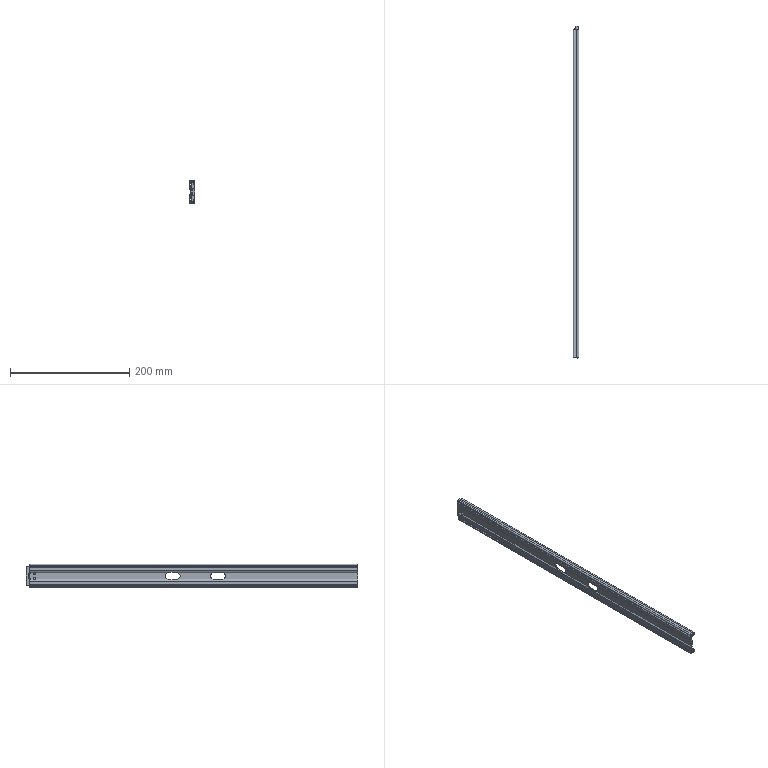Part | NX | features CENTERRAIL_5003_009_C-SRH51Y22 2 | 1 solid | 107 faces | box 9.386 x 557.2 x 40.224 mm | volume 63851 mm3 | plane 62 | cylinder 45 | commonest cylinder face diameters 1 x8 4 x6 2 x4 12 x4 0.2 x2 0.4 x2